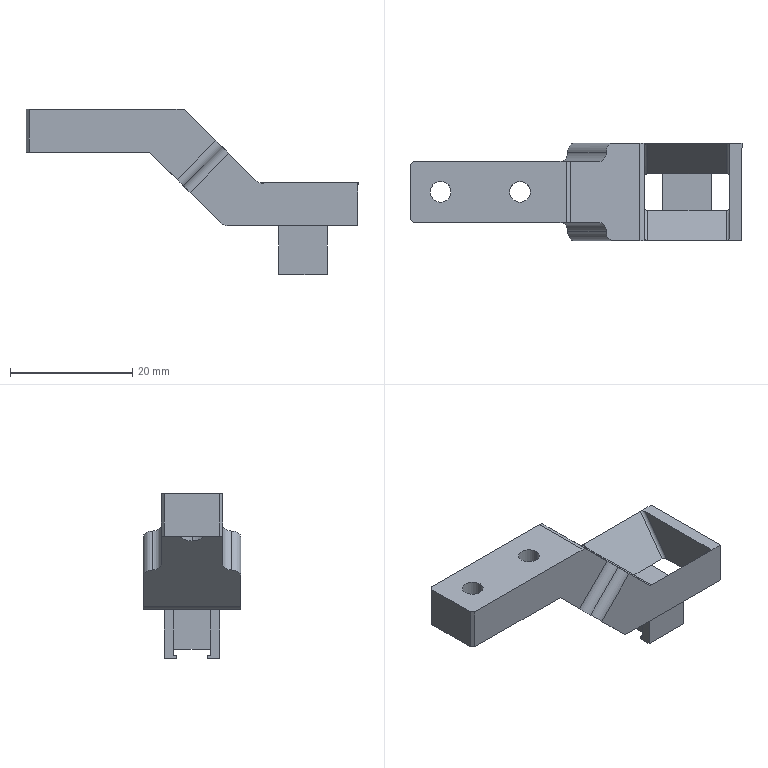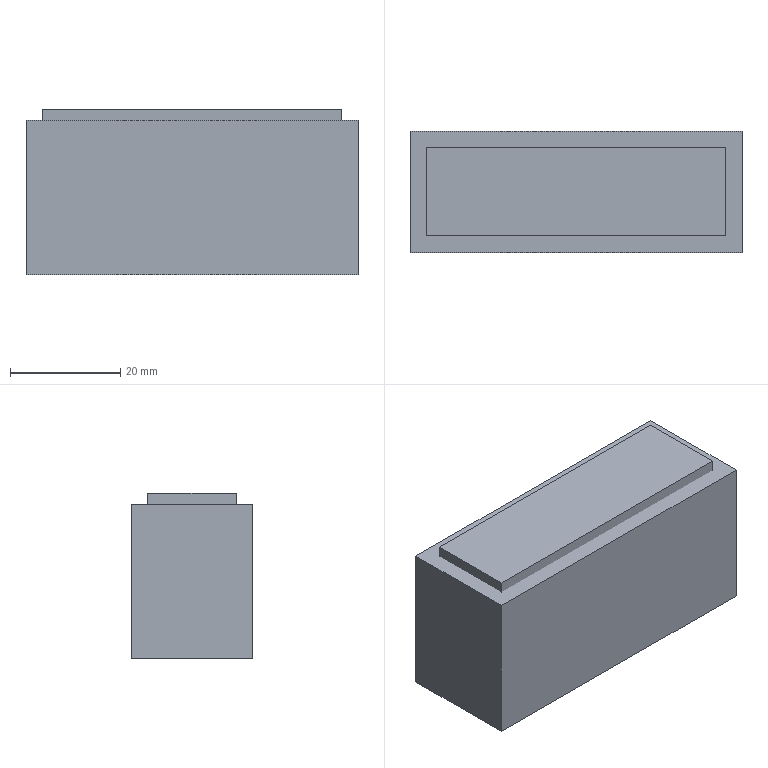CAM job | NX | 3-axis milling, drilling | part box 54.3 x 16 x 27 mm | stock box 60.3 x 22 x 30 mm
Tools:
number,name,description,diameter,corner_radius,flute_length,length,flutes
1,D63,Milling Tool-5 Parameters,63.0,0.0,50.0,75.0,2
10,D10,Milling Tool-5 Parameters,10.0,0.0,50.0,75.0,2
11,D10JING,Milling Tool-5 Parameters,10.0,0.0,50.0,75.0,2
5,D4R0.2,Milling Tool-5 Parameters,4.0,0.2,50.0,75.0,2
6,D6,Milling Tool-5 Parameters,6.0,0.0,50.0,75.0,2
8,D2R0.2,Milling Tool-5 Parameters,2.0,0.2,50.0,75.0,2
4,D4,Milling Tool-5 Parameters,4.0,0.0,50.0,75.0,2
7,D6A45,Milling Tool-5 Parameters,6.0,0.0,3.0,3.0,2
13,3.4ZT,Drilling Tool,3.4,0.0,35.0,50.0,2
Operations:
program,operation,operation_type,tool,method,geometry_group,spindle_rpm,surface_speed,feed_per_tooth,feed_cut,feed_plunge,cut_length_mm,path_length_mm,cut_time_min,machine_time_min
1,FLOOR_WALL,VolumeBased25DMillingOperation,D63,METHOD,A,6500.0,1286.0,0.0962,1250.0,100.0,135.3,189.3,0.1082,0.1136
1,DRILLING_COPY_1,Operation,D6A45,METHOD,A,5000.0,94.0,0.025,250.0,0.0,8.0,92.342,0.032,0.0404
1,DRILLING_COPY_COPY_1,Operation,3.4ZT,METHOD,A,2000.0,15.0,0.03,120.0,0.0,24.043,124.427,0.2004,0.2104
1,ADAPTIVE_MILLING,CavityMilling,D10,METHOD,A,9500.0,298.0,0.1579,3000.0,1000.0,4577.774,6777.93,1.543,1.763
1,ZLEVEL_PROFILE_COPY_COPY_1,ZLevelMilling,D10JING,METHOD,A,9500.0,298.0,0.0632,1200.0,100.0,351.256,541.95,0.2927,0.3118
1,ZLEVEL_PROFILE_COPY_COPY_1_COPY,ZLevelMilling,D10JING,METHOD,A,9500.0,298.0,0.0632,1200.0,100.0,102.608,251.142,0.0855,0.1004
1,ZLEVEL_PROFILE_COPY_COPY_1_COPY_COPY,ZLevelMilling,D6,METHOD,A,9500.0,298.0,0.0632,1200.0,100.0,71.317,236.997,0.0594,0.076
1,FLOOR_WALL_1,VolumeBased25DMillingOperation,D6,METHOD,A,9500.0,179.0,0.0658,1250.0,100.0,73.357,154.357,0.0587,0.0668
1,FIXED_CONTOUR,SurfaceContour,D6,METHOD,A,9500.0,179.0,0.1316,2500.0,500.0,761.324,844.253,0.325,0.3333
1,ZLEVEL_PROFILE_COPY_1,ZLevelMilling,D4R0.2,METHOD,A,9500.0,119.0,0.1053,2000.0,800.0,1361.071,1533.299,0.6844,0.7016
1,ZLEVEL_PROFILE_COPY_1_COPY_1,ZLevelMilling,D4R0.2,METHOD,A,9500.0,119.0,0.1053,2000.0,800.0,2499.604,2568.618,1.252,1.259
1,FIXED_CONTOUR_COPY,SurfaceContour,D4R0.2,METHOD,A,9500.0,59.0,0.1316,2500.0,500.0,3815.133,4326.027,1.643,1.694
1,ZLEVEL_PROFILE,ZLevelMilling,D4,METHOD,A,9500.0,119.0,0.1053,2000.0,800.0,835.798,1050.36,0.4681,0.4895
1,ZLEVEL_PROFILE_COPY,ZLevelMilling,D4,METHOD,A,9500.0,119.0,0.0632,1200.0,800.0,179.96,282.461,0.1768,0.1871
1,ZLEVEL_PROFILE_COPY_COPY,ZLevelMilling,D4,METHOD,A,9500.0,119.0,0.0632,1200.0,800.0,62.975,173.475,0.0684,0.0795
1,FIXED_CONTOUR_COPY_COPY,SurfaceContour,D2R0.2,METHOD,A,9500.0,59.0,0.1316,2500.0,500.0,4465.142,4990.921,1.886,1.938
1,ZLEVEL_PROFILE_COPY_1_COPY,ZLevelMilling,D2R0.2,METHOD,A,9500.0,119.0,0.1053,2000.0,800.0,1416.493,1746.296,0.7144,0.7474
1,ZLEVEL_PROFILE_1_COPY_1,ZLevelMilling,D6A45,METHOD,A,9500.0,179.0,0.0526,1000.0,100.0,84.34,285.699,0.0843,0.1045
2,FLOOR_WALL_COPY,VolumeBased25DMillingOperation,D63,METHOD,B,6500.0,1286.0,0.0962,1250.0,100.0,387.9,790.501,0.3103,0.3506
2,ADAPTIVE_MILLING_COPY,CavityMilling,D10,METHOD,B,9500.0,298.0,0.1579,3000.0,1000.0,2497.13,5051.483,0.8484,1.104
2,FLOOR_WALL_1_1,VolumeBased25DMillingOperation,D6,METHOD,B,9500.0,179.0,0.0658,1250.0,100.0,446.144,856.647,0.3569,0.398
2,ZLEVEL_PROFILE_COPY_1_COPY_2,ZLevelMilling,D4R0.2,METHOD,B,9500.0,119.0,0.1053,2000.0,800.0,2594.785,2679.794,1.299,1.308
2,HOLE_MILLING,CylinderMilling,D4,METHOD,B,9500.0,89.0,0.0658,1250.0,100.0,198.422,416.458,0.1587,0.1805
2,ZLEVEL_PROFILE_1_COPY_1_COPY_1,ZLevelMilling,D6A45,METHOD,B,9500.0,179.0,0.0526,1000.0,100.0,62.229,197.532,0.0622,0.0758
2,ZLEVEL_PROFILE_1_COPY_1_COPY_1_COPY,ZLevelMilling,D6A45,METHOD,B,9500.0,179.0,0.0526,1000.0,100.0,66.2,142.2,0.0662,0.0738
2,ZLEVEL_PROFILE_1_COPY_1_COPY_1_COPY_COPY,ZLevelMilling,D6A45,METHOD,B,9500.0,179.0,0.0526,1000.0,100.0,86.899,416.748,0.0869,0.1199